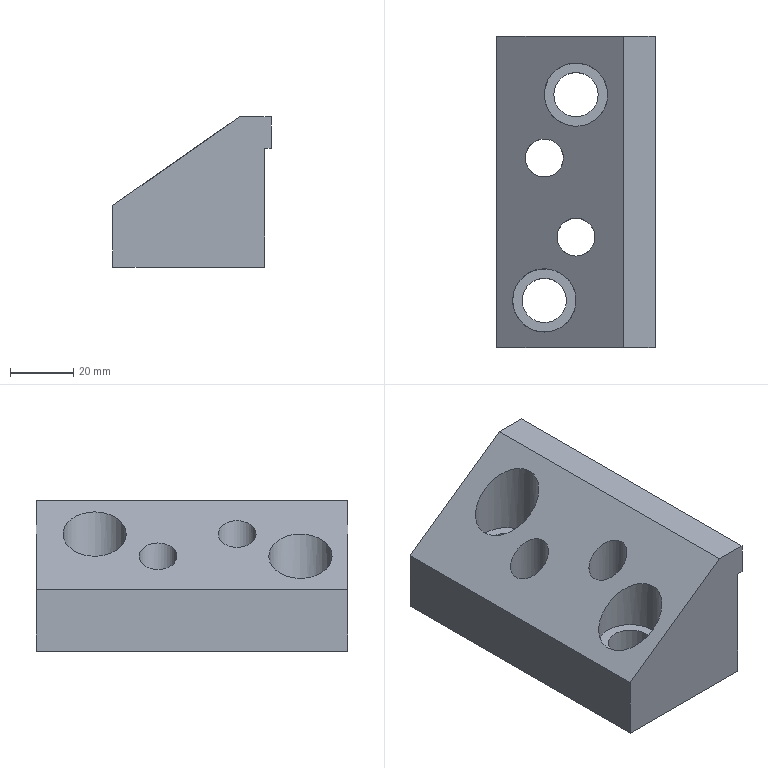Part | NX | features solid 2 | 1 solid | 17 faces | box 50 x 98.314 x 47.5 mm | volume 148836 mm3 | plane 11 | cylinder 6 | commonest cylinder face diameters 12 x2 14 x2 20 x2
STEP:
#1=CARTESIAN_POINT('',(-927.274,0.,-130.));
#2=VERTEX_POINT('',#1);
#3=CARTESIAN_POINT('',(-921.274,0.,-130.));
#4=DIRECTION('',(0.,0.,-1.));
#5=DIRECTION('',(-1.,0.,0.));
#6=AXIS2_PLACEMENT_3D('',#3,#4,#5);
#7=CIRCLE('',#6,6.);
#8=EDGE_CURVE('',#2,#2,#7,.F.);
#9=ORIENTED_EDGE('',*,*,#8,.T.);
#10=EDGE_LOOP('',(#9));
#11=FACE_BOUND('',#10,.T.);
#12=CARTESIAN_POINT('',(-928.274,-45.,-130.));
#13=VERTEX_POINT('',#12);
#14=CARTESIAN_POINT('',(-921.274,-45.,-130.));
#15=DIRECTION('',(0.,0.,-1.));
#16=DIRECTION('',(-1.,0.,0.));
#17=AXIS2_PLACEMENT_3D('',#14,#15,#16);
#18=CIRCLE('',#17,7.);
#19=EDGE_CURVE('',#13,#13,#18,.T.);
#20=ORIENTED_EDGE('',*,*,#19,.F.);
#21=EDGE_LOOP('',(#20));
#22=FACE_BOUND('',#21,.T.);
#23=CARTESIAN_POINT('',(-918.274,20.,-130.));
#24=VERTEX_POINT('',#23);
#25=CARTESIAN_POINT('',(-911.274,20.,-130.));
#26=DIRECTION('',(0.,0.,-1.));
#27=DIRECTION('',(-1.,0.,0.));
#28=AXIS2_PLACEMENT_3D('',#25,#26,#27);
#29=CIRCLE('',#28,7.);
#30=EDGE_CURVE('',#24,#24,#29,.T.);
#31=ORIENTED_EDGE('',*,*,#30,.F.);
#32=EDGE_LOOP('',(#31));
#33=FACE_BOUND('',#32,.T.);
#34=CARTESIAN_POINT('',(-888.274,38.416,-130.));
#35=VERTEX_POINT('',#34);
#36=CARTESIAN_POINT('',(-936.274,38.416,-130.));
#37=VERTEX_POINT('',#36);
#38=CARTESIAN_POINT('',(-896.274,38.416,-130.));
#39=DIRECTION('',(-1.,0.,0.));
#40=VECTOR('',#39,1000.);
#41=LINE('',#38,#40);
#42=EDGE_CURVE('',#35,#37,#41,.T.);
#43=ORIENTED_EDGE('',*,*,#42,.F.);
#44=CARTESIAN_POINT('',(-888.274,-59.897,-130.));
#45=VERTEX_POINT('',#44);
#46=CARTESIAN_POINT('',(-888.274,38.416,-130.));
#47=DIRECTION('',(0.,-1.,0.));
#48=VECTOR('',#47,1000.);
#49=LINE('',#46,#48);
#50=EDGE_CURVE('',#35,#45,#49,.T.);
#51=ORIENTED_EDGE('',*,*,#50,.T.);
#52=CARTESIAN_POINT('',(-936.274,-59.897,-130.));
#53=VERTEX_POINT('',#52);
#54=CARTESIAN_POINT('',(-896.274,-59.897,-130.));
#55=DIRECTION('',(-1.,0.,0.));
#56=VECTOR('',#55,1000.);
#57=LINE('',#54,#56);
#58=EDGE_CURVE('',#45,#53,#57,.T.);
#59=ORIENTED_EDGE('',*,*,#58,.T.);
#60=CARTESIAN_POINT('',(-936.274,38.416,-130.));
#61=DIRECTION('',(0.,-1.,0.));
#62=VECTOR('',#61,1000.);
#63=LINE('',#60,#62);
#64=EDGE_CURVE('',#37,#53,#63,.T.);
#65=ORIENTED_EDGE('',*,*,#64,.F.);
#66=EDGE_LOOP('',(#43,#51,#59,#65));
#67=FACE_BOUND('',#66,.T.);
#68=CARTESIAN_POINT('',(-917.274,-25.,-130.));
#69=VERTEX_POINT('',#68);
#70=CARTESIAN_POINT('',(-911.274,-25.,-130.));
#71=DIRECTION('',(0.,0.,-1.));
#72=DIRECTION('',(-1.,0.,0.));
#73=AXIS2_PLACEMENT_3D('',#70,#71,#72);
#74=CIRCLE('',#73,6.);
#75=EDGE_CURVE('',#69,#69,#74,.F.);
#76=ORIENTED_EDGE('',*,*,#75,.T.);
#77=EDGE_LOOP('',(#76));
#78=FACE_BOUND('',#77,.T.);
#79=CARTESIAN_POINT('',(-896.274,38.416,-130.));
#80=DIRECTION('',(0.,0.,-1.));
#81=DIRECTION('',(-1.,0.,0.));
#82=AXIS2_PLACEMENT_3D('',#79,#80,#81);
#83=PLANE('',#82);
#84=ADVANCED_FACE('',(#11,#22,#33,#67,#78),#83,.T.);
#85=CARTESIAN_POINT('',(-915.274,0.,-95.804));
#86=VERTEX_POINT('',#85);
#87=CARTESIAN_POINT('',(-921.274,0.,-100.005));
#88=DIRECTION('',(-0.5736,0.,0.8192));
#89=DIRECTION('',(0.8192,0.,0.5736));
#90=AXIS2_PLACEMENT_3D('',#87,#88,#89);
#91=ELLIPSE('',#90,7.325,6.);
#92=EDGE_CURVE('',#86,#86,#91,.F.);
#93=ORIENTED_EDGE('',*,*,#92,.T.);
#94=EDGE_LOOP('',(#93));
#95=FACE_BOUND('',#94,.T.);
#96=CARTESIAN_POINT('',(-911.274,-45.,-93.003));
#97=VERTEX_POINT('',#96);
#98=CARTESIAN_POINT('',(-921.274,-45.,-100.005));
#99=DIRECTION('',(-0.5736,0.,0.8192));
#100=DIRECTION('',(0.8192,0.,0.5736));
#101=AXIS2_PLACEMENT_3D('',#98,#99,#100);
#102=ELLIPSE('',#101,12.208,10.);
#103=EDGE_CURVE('',#97,#97,#102,.T.);
#104=ORIENTED_EDGE('',*,*,#103,.F.);
#105=EDGE_LOOP('',(#104));
#106=FACE_BOUND('',#105,.T.);
#107=CARTESIAN_POINT('',(-901.274,20.,-86.001));
#108=VERTEX_POINT('',#107);
#109=CARTESIAN_POINT('',(-911.274,20.,-93.003));
#110=DIRECTION('',(-0.5736,0.,0.8192));
#111=DIRECTION('',(0.8192,0.,0.5736));
#112=AXIS2_PLACEMENT_3D('',#109,#110,#111);
#113=ELLIPSE('',#112,12.208,10.);
#114=EDGE_CURVE('',#108,#108,#113,.T.);
#115=ORIENTED_EDGE('',*,*,#114,.F.);
#116=EDGE_LOOP('',(#115));
#117=FACE_BOUND('',#116,.T.);
#118=CARTESIAN_POINT('',(-936.274,38.416,-110.508));
#119=VERTEX_POINT('',#118);
#120=CARTESIAN_POINT('',(-936.274,-59.897,-110.508));
#121=VERTEX_POINT('',#120);
#122=CARTESIAN_POINT('',(-936.274,38.416,-110.508));
#123=DIRECTION('',(0.,-1.,0.));
#124=VECTOR('',#123,1000.);
#125=LINE('',#122,#124);
#126=EDGE_CURVE('',#119,#121,#125,.T.);
#127=ORIENTED_EDGE('',*,*,#126,.T.);
#128=CARTESIAN_POINT('',(-896.274,-59.897,-82.5));
#129=VERTEX_POINT('',#128);
#130=CARTESIAN_POINT('',(-896.274,-59.897,-82.5));
#131=DIRECTION('',(0.8192,0.,0.5736));
#132=VECTOR('',#131,1000.);
#133=LINE('',#130,#132);
#134=EDGE_CURVE('',#121,#129,#133,.T.);
#135=ORIENTED_EDGE('',*,*,#134,.T.);
#136=CARTESIAN_POINT('',(-896.274,38.416,-82.5));
#137=VERTEX_POINT('',#136);
#138=CARTESIAN_POINT('',(-896.274,38.416,-82.5));
#139=DIRECTION('',(0.,-1.,0.));
#140=VECTOR('',#139,1000.);
#141=LINE('',#138,#140);
#142=EDGE_CURVE('',#137,#129,#141,.T.);
#143=ORIENTED_EDGE('',*,*,#142,.F.);
#144=CARTESIAN_POINT('',(-896.274,38.416,-82.5));
#145=DIRECTION('',(0.8192,0.,0.5736));
#146=VECTOR('',#145,1000.);
#147=LINE('',#144,#146);
#148=EDGE_CURVE('',#119,#137,#147,.T.);
#149=ORIENTED_EDGE('',*,*,#148,.F.);
#150=EDGE_LOOP('',(#127,#135,#143,#149));
#151=FACE_BOUND('',#150,.T.);
#152=CARTESIAN_POINT('',(-905.274,-25.,-88.802));
#153=VERTEX_POINT('',#152);
#154=CARTESIAN_POINT('',(-911.274,-25.,-93.003));
#155=DIRECTION('',(-0.5736,0.,0.8192));
#156=DIRECTION('',(0.8192,0.,0.5736));
#157=AXIS2_PLACEMENT_3D('',#154,#155,#156);
#158=ELLIPSE('',#157,7.325,6.);
#159=EDGE_CURVE('',#153,#153,#158,.F.);
#160=ORIENTED_EDGE('',*,*,#159,.T.);
#161=EDGE_LOOP('',(#160));
#162=FACE_BOUND('',#161,.T.);
#163=CARTESIAN_POINT('',(-896.274,-59.897,-82.5));
#164=DIRECTION('',(-0.5736,0.,0.8192));
#165=DIRECTION('',(0.8192,0.,0.5736));
#166=AXIS2_PLACEMENT_3D('',#163,#164,#165);
#167=PLANE('',#166);
#168=ADVANCED_FACE('',(#95,#106,#117,#151,#162),#167,.T.);
#169=CARTESIAN_POINT('',(-888.274,-59.897,-92.5));
#170=VERTEX_POINT('',#169);
#171=CARTESIAN_POINT('',(-888.274,-59.897,-92.5));
#172=DIRECTION('',(0.,0.,-1.));
#173=VECTOR('',#172,1000.);
#174=LINE('',#171,#173);
#175=EDGE_CURVE('',#170,#45,#174,.T.);
#176=ORIENTED_EDGE('',*,*,#175,.F.);
#177=CARTESIAN_POINT('',(-886.274,-59.897,-92.5));
#178=VERTEX_POINT('',#177);
#179=CARTESIAN_POINT('',(-886.274,-59.897,-92.5));
#180=DIRECTION('',(-1.,0.,0.));
#181=VECTOR('',#180,1000.);
#182=LINE('',#179,#181);
#183=EDGE_CURVE('',#178,#170,#182,.T.);
#184=ORIENTED_EDGE('',*,*,#183,.F.);
#185=CARTESIAN_POINT('',(-886.274,-59.897,-82.5));
#186=VERTEX_POINT('',#185);
#187=CARTESIAN_POINT('',(-886.274,-59.897,-82.5));
#188=DIRECTION('',(0.,0.,-1.));
#189=VECTOR('',#188,1000.);
#190=LINE('',#187,#189);
#191=EDGE_CURVE('',#186,#178,#190,.T.);
#192=ORIENTED_EDGE('',*,*,#191,.F.);
#193=CARTESIAN_POINT('',(-886.274,-59.897,-82.5));
#194=DIRECTION('',(-1.,0.,0.));
#195=VECTOR('',#194,1000.);
#196=LINE('',#193,#195);
#197=EDGE_CURVE('',#186,#129,#196,.T.);
#198=ORIENTED_EDGE('',*,*,#197,.T.);
#199=ORIENTED_EDGE('',*,*,#134,.F.);
#200=CARTESIAN_POINT('',(-936.274,-59.897,-82.5));
#201=DIRECTION('',(0.,0.,-1.));
#202=VECTOR('',#201,1000.);
#203=LINE('',#200,#202);
#204=EDGE_CURVE('',#121,#53,#203,.T.);
#205=ORIENTED_EDGE('',*,*,#204,.T.);
#206=ORIENTED_EDGE('',*,*,#58,.F.);
#207=EDGE_LOOP('',(#176,#184,#192,#198,#199,#205,#206));
#208=FACE_BOUND('',#207,.T.);
#209=CARTESIAN_POINT('',(-896.274,-59.897,-82.5));
#210=DIRECTION('',(0.,1.,0.));
#211=DIRECTION('',(0.,0.,1.));
#212=AXIS2_PLACEMENT_3D('',#209,#210,#211);
#213=PLANE('',#212);
#214=ADVANCED_FACE('',(#208),#213,.F.);
#215=CARTESIAN_POINT('',(-886.274,38.416,-92.5));
#216=VERTEX_POINT('',#215);
#217=CARTESIAN_POINT('',(-888.274,38.416,-92.5));
#218=VERTEX_POINT('',#217);
#219=CARTESIAN_POINT('',(-886.274,38.416,-92.5));
#220=DIRECTION('',(-1.,0.,0.));
#221=VECTOR('',#220,1000.);
#222=LINE('',#219,#221);
#223=EDGE_CURVE('',#216,#218,#222,.T.);
#224=ORIENTED_EDGE('',*,*,#223,.T.);
#225=CARTESIAN_POINT('',(-888.274,38.416,-92.5));
#226=DIRECTION('',(0.,0.,-1.));
#227=VECTOR('',#226,1000.);
#228=LINE('',#225,#227);
#229=EDGE_CURVE('',#218,#35,#228,.T.);
#230=ORIENTED_EDGE('',*,*,#229,.T.);
#231=ORIENTED_EDGE('',*,*,#42,.T.);
#232=CARTESIAN_POINT('',(-936.274,38.416,-82.5));
#233=DIRECTION('',(0.,0.,1.));
#234=VECTOR('',#233,1000.);
#235=LINE('',#232,#234);
#236=EDGE_CURVE('',#119,#37,#235,.F.);
#237=ORIENTED_EDGE('',*,*,#236,.F.);
#238=ORIENTED_EDGE('',*,*,#148,.T.);
#239=CARTESIAN_POINT('',(-886.274,38.416,-82.5));
#240=VERTEX_POINT('',#239);
#241=CARTESIAN_POINT('',(-886.274,38.416,-82.5));
#242=DIRECTION('',(-1.,0.,0.));
#243=VECTOR('',#242,1000.);
#244=LINE('',#241,#243);
#245=EDGE_CURVE('',#240,#137,#244,.T.);
#246=ORIENTED_EDGE('',*,*,#245,.F.);
#247=CARTESIAN_POINT('',(-886.274,38.416,-82.5));
#248=DIRECTION('',(0.,0.,-1.));
#249=VECTOR('',#248,1000.);
#250=LINE('',#247,#249);
#251=EDGE_CURVE('',#240,#216,#250,.T.);
#252=ORIENTED_EDGE('',*,*,#251,.T.);
#253=EDGE_LOOP('',(#224,#230,#231,#237,#238,#246,#252));
#254=FACE_BOUND('',#253,.T.);
#255=CARTESIAN_POINT('',(-896.274,38.416,-82.5));
#256=DIRECTION('',(0.,1.,0.));
#257=DIRECTION('',(0.,0.,1.));
#258=AXIS2_PLACEMENT_3D('',#255,#256,#257);
#259=PLANE('',#258);
#260=ADVANCED_FACE('',(#254),#259,.T.);
#261=ORIENTED_EDGE('',*,*,#126,.F.);
#262=ORIENTED_EDGE('',*,*,#236,.T.);
#263=ORIENTED_EDGE('',*,*,#64,.T.);
#264=ORIENTED_EDGE('',*,*,#204,.F.);
#265=EDGE_LOOP('',(#261,#262,#263,#264));
#266=FACE_BOUND('',#265,.T.);
#267=CARTESIAN_POINT('',(-936.274,38.416,-82.5));
#268=DIRECTION('',(1.,0.,0.));
#269=DIRECTION('',(0.,0.,-1.));
#270=AXIS2_PLACEMENT_3D('',#267,#268,#269);
#271=PLANE('',#270);
#272=ADVANCED_FACE('',(#266),#271,.F.);
#273=ORIENTED_EDGE('',*,*,#197,.F.);
#274=CARTESIAN_POINT('',(-886.274,38.416,-82.5));
#275=DIRECTION('',(0.,-1.,0.));
#276=VECTOR('',#275,1000.);
#277=LINE('',#274,#276);
#278=EDGE_CURVE('',#240,#186,#277,.T.);
#279=ORIENTED_EDGE('',*,*,#278,.F.);
#280=ORIENTED_EDGE('',*,*,#245,.T.);
#281=ORIENTED_EDGE('',*,*,#142,.T.);
#282=EDGE_LOOP('',(#273,#279,#280,#281));
#283=FACE_BOUND('',#282,.T.);
#284=CARTESIAN_POINT('',(-886.274,38.416,-82.5));
#285=DIRECTION('',(0.,0.,1.));
#286=DIRECTION('',(0.,-1.,0.));
#287=AXIS2_PLACEMENT_3D('',#284,#285,#286);
#288=PLANE('',#287);
#289=ADVANCED_FACE('',(#283),#288,.T.);
#290=CARTESIAN_POINT('',(-886.274,38.416,-92.5));
#291=DIRECTION('',(0.,-1.,0.));
#292=VECTOR('',#291,1000.);
#293=LINE('',#290,#292);
#294=EDGE_CURVE('',#216,#178,#293,.T.);
#295=ORIENTED_EDGE('',*,*,#294,.F.);
#296=ORIENTED_EDGE('',*,*,#251,.F.);
#297=ORIENTED_EDGE('',*,*,#278,.T.);
#298=ORIENTED_EDGE('',*,*,#191,.T.);
#299=EDGE_LOOP('',(#295,#296,#297,#298));
#300=FACE_BOUND('',#299,.T.);
#301=CARTESIAN_POINT('',(-886.274,38.416,-82.5));
#302=DIRECTION('',(1.,0.,0.));
#303=DIRECTION('',(0.,0.,-1.));
#304=AXIS2_PLACEMENT_3D('',#301,#302,#303);
#305=PLANE('',#304);
#306=ADVANCED_FACE('',(#300),#305,.T.);
#307=ORIENTED_EDGE('',*,*,#294,.T.);
#308=ORIENTED_EDGE('',*,*,#183,.T.);
#309=CARTESIAN_POINT('',(-888.274,38.416,-92.5));
#310=DIRECTION('',(0.,1.,0.));
#311=VECTOR('',#310,1000.);
#312=LINE('',#309,#311);
#313=EDGE_CURVE('',#218,#170,#312,.F.);
#314=ORIENTED_EDGE('',*,*,#313,.F.);
#315=ORIENTED_EDGE('',*,*,#223,.F.);
#316=EDGE_LOOP('',(#307,#308,#314,#315));
#317=FACE_BOUND('',#316,.T.);
#318=CARTESIAN_POINT('',(-886.274,38.416,-92.5));
#319=DIRECTION('',(0.,0.,1.));
#320=DIRECTION('',(0.,-1.,0.));
#321=AXIS2_PLACEMENT_3D('',#318,#319,#320);
#322=PLANE('',#321);
#323=ADVANCED_FACE('',(#317),#322,.F.);
#324=ORIENTED_EDGE('',*,*,#229,.F.);
#325=ORIENTED_EDGE('',*,*,#313,.T.);
#326=ORIENTED_EDGE('',*,*,#175,.T.);
#327=ORIENTED_EDGE('',*,*,#50,.F.);
#328=EDGE_LOOP('',(#324,#325,#326,#327));
#329=FACE_BOUND('',#328,.T.);
#330=CARTESIAN_POINT('',(-888.274,38.416,-92.5));
#331=DIRECTION('',(1.,0.,0.));
#332=DIRECTION('',(0.,0.,-1.));
#333=AXIS2_PLACEMENT_3D('',#330,#331,#332);
#334=PLANE('',#333);
#335=ADVANCED_FACE('',(#329),#334,.T.);
#336=ORIENTED_EDGE('',*,*,#30,.T.);
#337=EDGE_LOOP('',(#336));
#338=FACE_BOUND('',#337,.T.);
#339=CARTESIAN_POINT('',(-918.274,20.,-110.));
#340=VERTEX_POINT('',#339);
#341=CARTESIAN_POINT('',(-911.274,20.,-110.));
#342=DIRECTION('',(0.,0.,-1.));
#343=DIRECTION('',(-1.,0.,0.));
#344=AXIS2_PLACEMENT_3D('',#341,#342,#343);
#345=CIRCLE('',#344,7.);
#346=EDGE_CURVE('',#340,#340,#345,.F.);
#347=ORIENTED_EDGE('',*,*,#346,.T.);
#348=EDGE_LOOP('',(#347));
#349=FACE_BOUND('',#348,.T.);
#350=CARTESIAN_POINT('',(-911.274,20.,-150.));
#351=DIRECTION('',(0.,0.,1.));
#352=DIRECTION('',(1.,0.,0.));
#353=AXIS2_PLACEMENT_3D('',#350,#351,#352);
#354=CYLINDRICAL_SURFACE('',#353,7.);
#355=ADVANCED_FACE('',(#338,#349),#354,.F.);
#356=ORIENTED_EDGE('',*,*,#346,.F.);
#357=EDGE_LOOP('',(#356));
#358=FACE_BOUND('',#357,.T.);
#359=CARTESIAN_POINT('',(-901.274,20.,-110.));
#360=VERTEX_POINT('',#359);
#361=CARTESIAN_POINT('',(-911.274,20.,-110.));
#362=DIRECTION('',(0.,0.,1.));
#363=DIRECTION('',(1.,0.,0.));
#364=AXIS2_PLACEMENT_3D('',#361,#362,#363);
#365=CIRCLE('',#364,10.);
#366=EDGE_CURVE('',#360,#360,#365,.T.);
#367=ORIENTED_EDGE('',*,*,#366,.T.);
#368=EDGE_LOOP('',(#367));
#369=FACE_BOUND('',#368,.T.);
#370=CARTESIAN_POINT('',(-911.274,20.,-110.));
#371=DIRECTION('',(0.,0.,-1.));
#372=DIRECTION('',(-1.,0.,0.));
#373=AXIS2_PLACEMENT_3D('',#370,#371,#372);
#374=PLANE('',#373);
#375=ADVANCED_FACE('',(#358,#369),#374,.F.);
#376=ORIENTED_EDGE('',*,*,#114,.T.);
#377=EDGE_LOOP('',(#376));
#378=FACE_BOUND('',#377,.T.);
#379=ORIENTED_EDGE('',*,*,#366,.F.);
#380=EDGE_LOOP('',(#379));
#381=FACE_BOUND('',#380,.T.);
#382=CARTESIAN_POINT('',(-911.274,20.,-110.));
#383=DIRECTION('',(0.,0.,1.));
#384=DIRECTION('',(1.,0.,0.));
#385=AXIS2_PLACEMENT_3D('',#382,#383,#384);
#386=CYLINDRICAL_SURFACE('',#385,10.);
#387=ADVANCED_FACE('',(#378,#381),#386,.F.);
#388=ORIENTED_EDGE('',*,*,#19,.T.);
#389=EDGE_LOOP('',(#388));
#390=FACE_BOUND('',#389,.T.);
#391=CARTESIAN_POINT('',(-928.274,-45.,-110.));
#392=VERTEX_POINT('',#391);
#393=CARTESIAN_POINT('',(-921.274,-45.,-110.));
#394=DIRECTION('',(0.,0.,-1.));
#395=DIRECTION('',(-1.,0.,0.));
#396=AXIS2_PLACEMENT_3D('',#393,#394,#395);
#397=CIRCLE('',#396,7.);
#398=EDGE_CURVE('',#392,#392,#397,.F.);
#399=ORIENTED_EDGE('',*,*,#398,.T.);
#400=EDGE_LOOP('',(#399));
#401=FACE_BOUND('',#400,.T.);
#402=CARTESIAN_POINT('',(-921.274,-45.,-150.));
#403=DIRECTION('',(0.,0.,1.));
#404=DIRECTION('',(1.,0.,0.));
#405=AXIS2_PLACEMENT_3D('',#402,#403,#404);
#406=CYLINDRICAL_SURFACE('',#405,7.);
#407=ADVANCED_FACE('',(#390,#401),#406,.F.);
#408=ORIENTED_EDGE('',*,*,#398,.F.);
#409=EDGE_LOOP('',(#408));
#410=FACE_BOUND('',#409,.T.);
#411=CARTESIAN_POINT('',(-911.274,-45.,-110.));
#412=VERTEX_POINT('',#411);
#413=CARTESIAN_POINT('',(-921.274,-45.,-110.));
#414=DIRECTION('',(0.,0.,1.));
#415=DIRECTION('',(1.,0.,0.));
#416=AXIS2_PLACEMENT_3D('',#413,#414,#415);
#417=CIRCLE('',#416,10.);
#418=EDGE_CURVE('',#412,#412,#417,.T.);
#419=ORIENTED_EDGE('',*,*,#418,.T.);
#420=EDGE_LOOP('',(#419));
#421=FACE_BOUND('',#420,.T.);
#422=CARTESIAN_POINT('',(-921.274,-45.,-110.));
#423=DIRECTION('',(0.,0.,-1.));
#424=DIRECTION('',(-1.,0.,0.));
#425=AXIS2_PLACEMENT_3D('',#422,#423,#424);
#426=PLANE('',#425);
#427=ADVANCED_FACE('',(#410,#421),#426,.F.);
#428=ORIENTED_EDGE('',*,*,#103,.T.);
#429=EDGE_LOOP('',(#428));
#430=FACE_BOUND('',#429,.T.);
#431=ORIENTED_EDGE('',*,*,#418,.F.);
#432=EDGE_LOOP('',(#431));
#433=FACE_BOUND('',#432,.T.);
#434=CARTESIAN_POINT('',(-921.274,-45.,-110.));
#435=DIRECTION('',(0.,0.,1.));
#436=DIRECTION('',(1.,0.,0.));
#437=AXIS2_PLACEMENT_3D('',#434,#435,#436);
#438=CYLINDRICAL_SURFACE('',#437,10.);
#439=ADVANCED_FACE('',(#430,#433),#438,.F.);
#440=ORIENTED_EDGE('',*,*,#8,.F.);
#441=EDGE_LOOP('',(#440));
#442=FACE_BOUND('',#441,.T.);
#443=ORIENTED_EDGE('',*,*,#92,.F.);
#444=EDGE_LOOP('',(#443));
#445=FACE_BOUND('',#444,.T.);
#446=CARTESIAN_POINT('',(-921.274,0.,-160.));
#447=DIRECTION('',(0.,0.,1.));
#448=DIRECTION('',(1.,0.,0.));
#449=AXIS2_PLACEMENT_3D('',#446,#447,#448);
#450=CYLINDRICAL_SURFACE('',#449,6.);
#451=ADVANCED_FACE('',(#442,#445),#450,.F.);
#452=ORIENTED_EDGE('',*,*,#75,.F.);
#453=EDGE_LOOP('',(#452));
#454=FACE_BOUND('',#453,.T.);
#455=ORIENTED_EDGE('',*,*,#159,.F.);
#456=EDGE_LOOP('',(#455));
#457=FACE_BOUND('',#456,.T.);
#458=CARTESIAN_POINT('',(-911.274,-25.,-160.));
#459=DIRECTION('',(0.,0.,1.));
#460=DIRECTION('',(1.,0.,0.));
#461=AXIS2_PLACEMENT_3D('',#458,#459,#460);
#462=CYLINDRICAL_SURFACE('',#461,6.);
#463=ADVANCED_FACE('',(#454,#457),#462,.F.);
#464=CLOSED_SHELL('',(#84,#168,#214,#260,#272,#289,#306,#323,#335,#355,#375,#387,#407,#427,#439,#451,#463));
#465=MANIFOLD_SOLID_BREP('',#464);
#466=(LENGTH_UNIT()NAMED_UNIT(*)SI_UNIT(.MILLI.,.METRE.));
#467=UNCERTAINTY_MEASURE_WITH_UNIT(LENGTH_MEASURE(0.00001),#466,'','');
#468=(NAMED_UNIT(*)PLANE_ANGLE_UNIT()SI_UNIT($,.RADIAN.));
#469=(NAMED_UNIT(*)SI_UNIT($,.STERADIAN.)SOLID_ANGLE_UNIT());
#470=(GEOMETRIC_REPRESENTATION_CONTEXT(3)GLOBAL_UNCERTAINTY_ASSIGNED_CONTEXT((#467))GLOBAL_UNIT_ASSIGNED_CONTEXT((#466,#468,#469))REPRESENTATION_CONTEXT('',''));
#471=ADVANCED_BREP_SHAPE_REPRESENTATION('',(#465),#470);